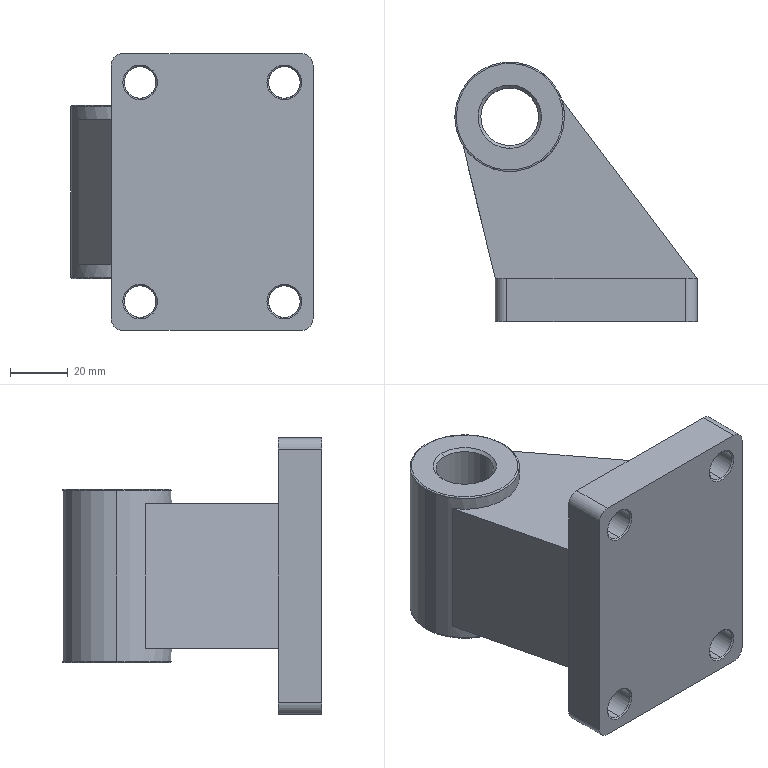Part | STEP file | _F-SI100CR(SE) | 1 solid | 65 faces | box 84 x 90 x 96 mm | volume 270895 mm3 | cylinder 24 | cone 20 | plane 17 | spline 4 | commonest cylinder face diameters 11 x8 18 x8 8 x4 20 x2 38 x2